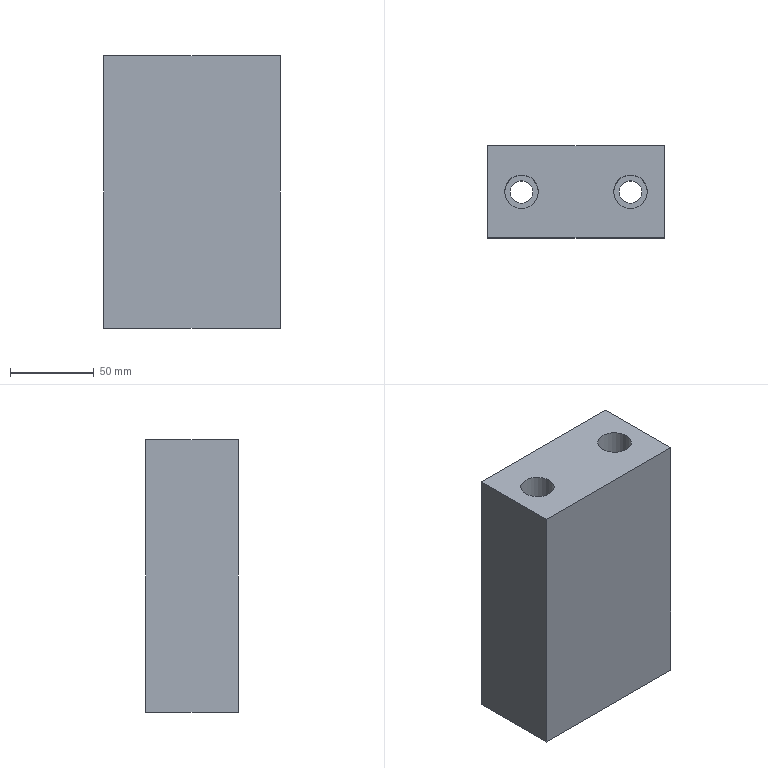Part | STEP file | lll_id4198_x_t | 1 solid | 12 faces | box 105 x 55 x 162.5 mm | volume 862331 mm3 | plane 8 | cylinder 4 | commonest cylinder face diameters 13.5 x2 20 x2
STEP:
#1=CARTESIAN_POINT('',(2207.435,-414.,82.5));
#2=VERTEX_POINT('',#1);
#3=CARTESIAN_POINT('',(2102.435,-414.,82.5));
#4=VERTEX_POINT('',#3);
#5=CARTESIAN_POINT('',(2137.435,-414.,82.5));
#6=DIRECTION('',(-1.,0.,0.));
#7=VECTOR('',#6,1.);
#8=LINE('',#5,#7);
#9=EDGE_CURVE('',#2,#4,#8,.T.);
#10=ORIENTED_EDGE('',*,*,#9,.F.);
#11=CARTESIAN_POINT('',(2207.435,-359.,82.5));
#12=VERTEX_POINT('',#11);
#13=CARTESIAN_POINT('',(2207.435,-384.,82.5));
#14=DIRECTION('',(0.,-1.,0.));
#15=VECTOR('',#14,1.);
#16=LINE('',#13,#15);
#17=EDGE_CURVE('',#12,#2,#16,.T.);
#18=ORIENTED_EDGE('',*,*,#17,.F.);
#19=CARTESIAN_POINT('',(2102.435,-359.,82.5));
#20=VERTEX_POINT('',#19);
#21=CARTESIAN_POINT('',(2137.435,-359.,82.5));
#22=DIRECTION('',(1.,0.,0.));
#23=VECTOR('',#22,1.);
#24=LINE('',#21,#23);
#25=EDGE_CURVE('',#20,#12,#24,.T.);
#26=ORIENTED_EDGE('',*,*,#25,.F.);
#27=CARTESIAN_POINT('',(2102.435,-384.,82.5));
#28=DIRECTION('',(0.,1.,0.));
#29=VECTOR('',#28,1.);
#30=LINE('',#27,#29);
#31=EDGE_CURVE('',#4,#20,#30,.T.);
#32=ORIENTED_EDGE('',*,*,#31,.F.);
#33=EDGE_LOOP('',(#10,#18,#26,#32));
#34=FACE_BOUND('',#33,.T.);
#35=CARTESIAN_POINT('',(2112.435,-386.5,82.5));
#36=VERTEX_POINT('',#35);
#37=CARTESIAN_POINT('',(2122.435,-386.5,82.5));
#38=DIRECTION('',(0.,0.,1.));
#39=DIRECTION('',(-1.,0.,0.));
#40=AXIS2_PLACEMENT_3D('',#37,#38,#39);
#41=CIRCLE('',#40,10.);
#42=EDGE_CURVE('',#36,#36,#41,.T.);
#43=ORIENTED_EDGE('',*,*,#42,.F.);
#44=EDGE_LOOP('',(#43));
#45=FACE_BOUND('',#44,.T.);
#46=CARTESIAN_POINT('',(2177.435,-386.5,82.5));
#47=VERTEX_POINT('',#46);
#48=CARTESIAN_POINT('',(2187.435,-386.5,82.5));
#49=DIRECTION('',(0.,0.,-1.));
#50=DIRECTION('',(-1.,0.,0.));
#51=AXIS2_PLACEMENT_3D('',#48,#49,#50);
#52=CIRCLE('',#51,10.);
#53=EDGE_CURVE('',#47,#47,#52,.T.);
#54=ORIENTED_EDGE('',*,*,#53,.T.);
#55=EDGE_LOOP('',(#54));
#56=FACE_BOUND('',#55,.T.);
#57=CARTESIAN_POINT('',(2690.435,3.,82.5));
#58=DIRECTION('',(0.,0.,-1.));
#59=DIRECTION('',(-1.,0.,0.));
#60=AXIS2_PLACEMENT_3D('',#57,#58,#59);
#61=PLANE('',#60);
#62=ADVANCED_FACE('',(#34,#45,#56),#61,.F.);
#63=CARTESIAN_POINT('',(2180.685,-386.5,-80.));
#64=VERTEX_POINT('',#63);
#65=CARTESIAN_POINT('',(2187.435,-386.5,-80.));
#66=DIRECTION('',(0.,0.,-1.));
#67=DIRECTION('',(-1.,0.,0.));
#68=AXIS2_PLACEMENT_3D('',#65,#66,#67);
#69=CIRCLE('',#68,6.75);
#70=EDGE_CURVE('',#64,#64,#69,.T.);
#71=ORIENTED_EDGE('',*,*,#70,.F.);
#72=EDGE_LOOP('',(#71));
#73=FACE_BOUND('',#72,.T.);
#74=CARTESIAN_POINT('',(2207.435,-414.,-80.));
#75=VERTEX_POINT('',#74);
#76=CARTESIAN_POINT('',(2207.435,-359.,-80.));
#77=VERTEX_POINT('',#76);
#78=CARTESIAN_POINT('',(2207.435,-384.,-80.));
#79=DIRECTION('',(0.,1.,0.));
#80=VECTOR('',#79,1.);
#81=LINE('',#78,#80);
#82=EDGE_CURVE('',#75,#77,#81,.T.);
#83=ORIENTED_EDGE('',*,*,#82,.F.);
#84=CARTESIAN_POINT('',(2102.435,-414.,-80.));
#85=VERTEX_POINT('',#84);
#86=CARTESIAN_POINT('',(2137.435,-414.,-80.));
#87=DIRECTION('',(1.,0.,0.));
#88=VECTOR('',#87,1.);
#89=LINE('',#86,#88);
#90=EDGE_CURVE('',#85,#75,#89,.T.);
#91=ORIENTED_EDGE('',*,*,#90,.F.);
#92=CARTESIAN_POINT('',(2102.435,-359.,-80.));
#93=VERTEX_POINT('',#92);
#94=CARTESIAN_POINT('',(2102.435,-384.,-80.));
#95=DIRECTION('',(0.,-1.,0.));
#96=VECTOR('',#95,1.);
#97=LINE('',#94,#96);
#98=EDGE_CURVE('',#93,#85,#97,.T.);
#99=ORIENTED_EDGE('',*,*,#98,.F.);
#100=CARTESIAN_POINT('',(2137.435,-359.,-80.));
#101=DIRECTION('',(-1.,0.,0.));
#102=VECTOR('',#101,1.);
#103=LINE('',#100,#102);
#104=EDGE_CURVE('',#77,#93,#103,.T.);
#105=ORIENTED_EDGE('',*,*,#104,.F.);
#106=EDGE_LOOP('',(#83,#91,#99,#105));
#107=FACE_BOUND('',#106,.T.);
#108=CARTESIAN_POINT('',(2115.685,-386.5,-80.));
#109=VERTEX_POINT('',#108);
#110=CARTESIAN_POINT('',(2122.435,-386.5,-80.));
#111=DIRECTION('',(0.,0.,1.));
#112=DIRECTION('',(-1.,0.,0.));
#113=AXIS2_PLACEMENT_3D('',#110,#111,#112);
#114=CIRCLE('',#113,6.75);
#115=EDGE_CURVE('',#109,#109,#114,.T.);
#116=ORIENTED_EDGE('',*,*,#115,.T.);
#117=EDGE_LOOP('',(#116));
#118=FACE_BOUND('',#117,.T.);
#119=CARTESIAN_POINT('',(2137.435,-384.,-80.));
#120=DIRECTION('',(0.,0.,-1.));
#121=DIRECTION('',(-1.,0.,0.));
#122=AXIS2_PLACEMENT_3D('',#119,#120,#121);
#123=PLANE('',#122);
#124=ADVANCED_FACE('',(#73,#107,#118),#123,.T.);
#125=CARTESIAN_POINT('',(2207.435,-414.,-80.));
#126=DIRECTION('',(0.,0.,1.));
#127=VECTOR('',#126,1.);
#128=LINE('',#125,#127);
#129=EDGE_CURVE('',#75,#2,#128,.T.);
#130=ORIENTED_EDGE('',*,*,#129,.T.);
#131=ORIENTED_EDGE('',*,*,#9,.T.);
#132=CARTESIAN_POINT('',(2102.435,-414.,-80.));
#133=DIRECTION('',(0.,0.,1.));
#134=VECTOR('',#133,1.);
#135=LINE('',#132,#134);
#136=EDGE_CURVE('',#85,#4,#135,.T.);
#137=ORIENTED_EDGE('',*,*,#136,.F.);
#138=ORIENTED_EDGE('',*,*,#90,.T.);
#139=EDGE_LOOP('',(#130,#131,#137,#138));
#140=FACE_OUTER_BOUND('',#139,.T.);
#141=CARTESIAN_POINT('',(2137.435,-414.,-80.));
#142=DIRECTION('',(0.,-1.,0.));
#143=DIRECTION('',(0.,0.,-1.));
#144=AXIS2_PLACEMENT_3D('',#141,#142,#143);
#145=PLANE('',#144);
#146=ADVANCED_FACE('',(#140),#145,.T.);
#147=ORIENTED_EDGE('',*,*,#136,.T.);
#148=ORIENTED_EDGE('',*,*,#31,.T.);
#149=CARTESIAN_POINT('',(2102.435,-359.,-80.));
#150=DIRECTION('',(0.,0.,1.));
#151=VECTOR('',#150,1.);
#152=LINE('',#149,#151);
#153=EDGE_CURVE('',#93,#20,#152,.T.);
#154=ORIENTED_EDGE('',*,*,#153,.F.);
#155=ORIENTED_EDGE('',*,*,#98,.T.);
#156=EDGE_LOOP('',(#147,#148,#154,#155));
#157=FACE_OUTER_BOUND('',#156,.T.);
#158=CARTESIAN_POINT('',(2102.435,-384.,-80.));
#159=DIRECTION('',(-1.,0.,0.));
#160=DIRECTION('',(0.,0.,1.));
#161=AXIS2_PLACEMENT_3D('',#158,#159,#160);
#162=PLANE('',#161);
#163=ADVANCED_FACE('',(#157),#162,.T.);
#164=ORIENTED_EDGE('',*,*,#153,.T.);
#165=ORIENTED_EDGE('',*,*,#25,.T.);
#166=CARTESIAN_POINT('',(2207.435,-359.,-80.));
#167=DIRECTION('',(0.,0.,1.));
#168=VECTOR('',#167,1.);
#169=LINE('',#166,#168);
#170=EDGE_CURVE('',#77,#12,#169,.T.);
#171=ORIENTED_EDGE('',*,*,#170,.F.);
#172=ORIENTED_EDGE('',*,*,#104,.T.);
#173=EDGE_LOOP('',(#164,#165,#171,#172));
#174=FACE_OUTER_BOUND('',#173,.T.);
#175=CARTESIAN_POINT('',(2137.435,-359.,-80.));
#176=DIRECTION('',(0.,1.,0.));
#177=DIRECTION('',(0.,0.,1.));
#178=AXIS2_PLACEMENT_3D('',#175,#176,#177);
#179=PLANE('',#178);
#180=ADVANCED_FACE('',(#174),#179,.T.);
#181=ORIENTED_EDGE('',*,*,#82,.T.);
#182=ORIENTED_EDGE('',*,*,#170,.T.);
#183=ORIENTED_EDGE('',*,*,#17,.T.);
#184=ORIENTED_EDGE('',*,*,#129,.F.);
#185=EDGE_LOOP('',(#181,#182,#183,#184));
#186=FACE_OUTER_BOUND('',#185,.T.);
#187=CARTESIAN_POINT('',(2207.435,-384.,-80.));
#188=DIRECTION('',(1.,0.,0.));
#189=DIRECTION('',(0.,0.,-1.));
#190=AXIS2_PLACEMENT_3D('',#187,#188,#189);
#191=PLANE('',#190);
#192=ADVANCED_FACE('',(#186),#191,.T.);
#193=CARTESIAN_POINT('',(2112.435,-386.5,-4.));
#194=VERTEX_POINT('',#193);
#195=CARTESIAN_POINT('',(2122.435,-386.5,-4.));
#196=DIRECTION('',(0.,0.,-1.));
#197=DIRECTION('',(-1.,0.,0.));
#198=AXIS2_PLACEMENT_3D('',#195,#196,#197);
#199=CIRCLE('',#198,10.);
#200=EDGE_CURVE('',#194,#194,#199,.T.);
#201=ORIENTED_EDGE('',*,*,#200,.T.);
#202=EDGE_LOOP('',(#201));
#203=FACE_BOUND('',#202,.T.);
#204=ORIENTED_EDGE('',*,*,#42,.T.);
#205=EDGE_LOOP('',(#204));
#206=FACE_BOUND('',#205,.T.);
#207=CARTESIAN_POINT('',(2122.435,-386.5,3.2));
#208=DIRECTION('',(0.,0.,-1.));
#209=DIRECTION('',(1.,0.,0.));
#210=AXIS2_PLACEMENT_3D('',#207,#208,#209);
#211=CYLINDRICAL_SURFACE('',#210,10.);
#212=ADVANCED_FACE('',(#203,#206),#211,.F.);
#213=ORIENTED_EDGE('',*,*,#115,.F.);
#214=EDGE_LOOP('',(#213));
#215=FACE_BOUND('',#214,.T.);
#216=CARTESIAN_POINT('',(2115.685,-386.5,-4.));
#217=VERTEX_POINT('',#216);
#218=CARTESIAN_POINT('',(2122.435,-386.5,-4.));
#219=DIRECTION('',(0.,0.,-1.));
#220=DIRECTION('',(-1.,0.,0.));
#221=AXIS2_PLACEMENT_3D('',#218,#219,#220);
#222=CIRCLE('',#221,6.75);
#223=EDGE_CURVE('',#217,#217,#222,.T.);
#224=ORIENTED_EDGE('',*,*,#223,.F.);
#225=EDGE_LOOP('',(#224));
#226=FACE_BOUND('',#225,.T.);
#227=CARTESIAN_POINT('',(2122.435,-386.5,-96.8));
#228=DIRECTION('',(0.,0.,-1.));
#229=DIRECTION('',(1.,0.,0.));
#230=AXIS2_PLACEMENT_3D('',#227,#228,#229);
#231=CYLINDRICAL_SURFACE('',#230,6.75);
#232=ADVANCED_FACE('',(#215,#226),#231,.F.);
#233=ORIENTED_EDGE('',*,*,#223,.T.);
#234=EDGE_LOOP('',(#233));
#235=FACE_BOUND('',#234,.T.);
#236=ORIENTED_EDGE('',*,*,#200,.F.);
#237=EDGE_LOOP('',(#236));
#238=FACE_BOUND('',#237,.T.);
#239=CARTESIAN_POINT('',(2122.435,-386.5,-4.));
#240=DIRECTION('',(0.,0.,-1.));
#241=DIRECTION('',(1.,0.,0.));
#242=AXIS2_PLACEMENT_3D('',#239,#240,#241);
#243=PLANE('',#242);
#244=ADVANCED_FACE('',(#235,#238),#243,.F.);
#245=CARTESIAN_POINT('',(2177.435,-386.5,-4.));
#246=VERTEX_POINT('',#245);
#247=CARTESIAN_POINT('',(2187.435,-386.5,-4.));
#248=DIRECTION('',(0.,0.,1.));
#249=DIRECTION('',(-1.,0.,0.));
#250=AXIS2_PLACEMENT_3D('',#247,#248,#249);
#251=CIRCLE('',#250,10.);
#252=EDGE_CURVE('',#246,#246,#251,.T.);
#253=ORIENTED_EDGE('',*,*,#252,.F.);
#254=EDGE_LOOP('',(#253));
#255=FACE_BOUND('',#254,.T.);
#256=ORIENTED_EDGE('',*,*,#53,.F.);
#257=EDGE_LOOP('',(#256));
#258=FACE_BOUND('',#257,.T.);
#259=CARTESIAN_POINT('',(2187.435,-386.5,3.2));
#260=DIRECTION('',(0.,0.,-1.));
#261=DIRECTION('',(-1.,0.,0.));
#262=AXIS2_PLACEMENT_3D('',#259,#260,#261);
#263=CYLINDRICAL_SURFACE('',#262,10.);
#264=ADVANCED_FACE('',(#255,#258),#263,.F.);
#265=ORIENTED_EDGE('',*,*,#70,.T.);
#266=EDGE_LOOP('',(#265));
#267=FACE_BOUND('',#266,.T.);
#268=CARTESIAN_POINT('',(2180.685,-386.5,-4.));
#269=VERTEX_POINT('',#268);
#270=CARTESIAN_POINT('',(2187.435,-386.5,-4.));
#271=DIRECTION('',(0.,0.,1.));
#272=DIRECTION('',(-1.,0.,0.));
#273=AXIS2_PLACEMENT_3D('',#270,#271,#272);
#274=CIRCLE('',#273,6.75);
#275=EDGE_CURVE('',#269,#269,#274,.T.);
#276=ORIENTED_EDGE('',*,*,#275,.T.);
#277=EDGE_LOOP('',(#276));
#278=FACE_BOUND('',#277,.T.);
#279=CARTESIAN_POINT('',(2187.435,-386.5,-96.8));
#280=DIRECTION('',(0.,0.,-1.));
#281=DIRECTION('',(-1.,0.,0.));
#282=AXIS2_PLACEMENT_3D('',#279,#280,#281);
#283=CYLINDRICAL_SURFACE('',#282,6.75);
#284=ADVANCED_FACE('',(#267,#278),#283,.F.);
#285=ORIENTED_EDGE('',*,*,#275,.F.);
#286=EDGE_LOOP('',(#285));
#287=FACE_BOUND('',#286,.T.);
#288=ORIENTED_EDGE('',*,*,#252,.T.);
#289=EDGE_LOOP('',(#288));
#290=FACE_BOUND('',#289,.T.);
#291=CARTESIAN_POINT('',(2187.435,-386.5,-4.));
#292=DIRECTION('',(0.,0.,-1.));
#293=DIRECTION('',(-1.,0.,0.));
#294=AXIS2_PLACEMENT_3D('',#291,#292,#293);
#295=PLANE('',#294);
#296=ADVANCED_FACE('',(#287,#290),#295,.F.);
#297=CLOSED_SHELL('',(#62,#124,#146,#163,#180,#192,#212,#232,#244,#264,#284,#296));
#298=MANIFOLD_SOLID_BREP('',#297);
#299=(LENGTH_UNIT()NAMED_UNIT(*)SI_UNIT(.MILLI.,.METRE.));
#300=UNCERTAINTY_MEASURE_WITH_UNIT(LENGTH_MEASURE(0.00002),#299,'','');
#301=(NAMED_UNIT(*)PLANE_ANGLE_UNIT()SI_UNIT($,.RADIAN.));
#302=PLANE_ANGLE_MEASURE_WITH_UNIT(PLANE_ANGLE_MEASURE(0.01745),#301);
#303=DIMENSIONAL_EXPONENTS(0.,0.,0.,0.,0.,0.,0.);
#304=(CONVERSION_BASED_UNIT('DEGREE',#302)NAMED_UNIT(#303)PLANE_ANGLE_UNIT());
#305=(NAMED_UNIT(*)SI_UNIT($,.STERADIAN.)SOLID_ANGLE_UNIT());
#306=(GEOMETRIC_REPRESENTATION_CONTEXT(3)GLOBAL_UNCERTAINTY_ASSIGNED_CONTEXT((#300))GLOBAL_UNIT_ASSIGNED_CONTEXT((#299,#304,#305))REPRESENTATION_CONTEXT('',''));
#307=ADVANCED_BREP_SHAPE_REPRESENTATION('',(#298),#306);